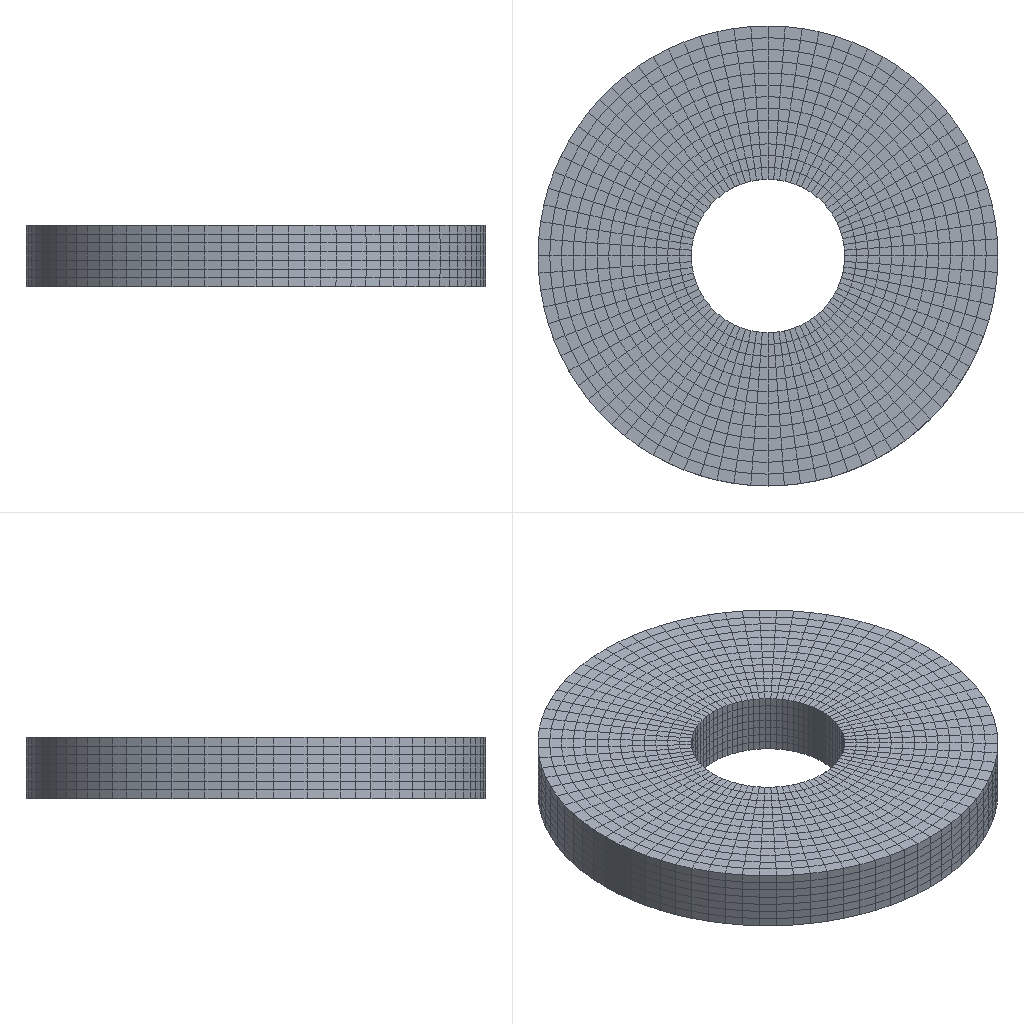Simulation study | abaqus
Set-up summary:
category,name,step,type,value,unit,region
solver,abaqus
solver,version,,,Abaqus/Standard 2020
units,not stated in the deck,,not stated
analysis,deck,,static,static
load_step,Step-1,Step-1,static
load_step,requested,,,1
mesh,nodes,,,10800
mesh,elements,,,9019
element_type,C3D8,,solid,7735
element_type,R3D3,,rigid,14
element_type,R3D4,,rigid,1270
load,load commands in deck,,count,1
bc,support commands in deck,,count,1
material,MATERIAL-1,,in results
material,MATERIAL-1-COPY,,in results
check,setup vs results,,match,"per instance, exact: element labels, types and connectivity; labels of the nodes the elements use; coordinates of those nodes at SINGLE_PRECISION in 2 of 2 instance(s)"
Abaqus input file, long lists of numbers shortened:
*Heading
** Job name: Job-1 Model name: Model-1
** Generated by: Abaqus/CAE 2020
*Preprint, echo=NO, model=NO, history=NO, contact=NO
**
** PARTS
**
*Part, name=Part-1
*Node
      1,   1.118,  -2.236,           4.
      2,   1.118,  -2.236,           0.
** (1277 more lines like these left out)
*Element, type=R3D4
  1,   1,   3, 105, 156
  2,   3,   4, 106, 105
** (1268 more lines like these left out)
*Element, type=R3D3
677,  963,  757,  736
678,  987,  863,  818
** (12 more lines like these left out)
*Node
   1280,           0., -1.5308085e-16,           4.
*Nset, nset=Part-1-RefPt_, internal
1280,
*Elset, elset=Part-1, generate
    1,  1284,     1
*End Part
**
*Part, name=Part-2
*Node
      1,           0.,         -2.5,           2.
      2,           0.,         -7.5,           2.
** (9518 more lines like these left out)
*Element, type=C3D8
   1,    1,   21,  485,   56,   97, 1133, 3689,  886
   2,   21,   22,  486,  485, 1133, 1134, 3690, 3689
** (7733 more lines like these left out)
*Nset, nset=Set-3, generate
    1,  9520,     1
*Elset, elset=Set-3, generate
    1,  7735,     1
** Section: Section-1
*Solid Section, elset=Set-3, material=Material-1
,
*End Part
**
*Part, name=crack2
*End Part
**
**
** ASSEMBLY
**
*Assembly, name=Assembly
**
*Instance, name=Part-1-1, part=Part-1
*End Instance
**
*Instance, name=Part-2-1, part=Part-2
          0.,           0.,           1.
*End Instance
**
*Instance, name=crack2-1, part=crack2
        2.46,         0.05,           2.
*End Instance
**
*Nset, nset=Set-1, instance=Part-1-1
    1,    2,    3,    4,    5,    6,    7,    8,    9,   10,   11,   12,   13,   14,   15,   16
   17,   18,   19,   20,   21,   22,   23,   24,   25,   26,   27,   28,   29,   30,   31,   32
** (39 more lines like these left out)
*Elset, elset=Set-1, instance=Part-1-1, generate
  677,  1284,     1
*Nset, nset=Set-2, instance=Part-1-1
 1280,
*Nset, nset=_PickedSet19, internal, instance=Part-2-1, generate
    1,  9520,     1
*Elset, elset=_PickedSet19, internal, instance=Part-2-1, generate
    1,  7735,     1
*Elset, elset=_Surf-6_S4, internal, instance=Part-2-1, generate
   13,  7735,    13
*Surface, type=ELEMENT, name=Surf-6
_Surf-6_S4, S4
*Elset, elset=_m_Surf-1_SPOS, internal, instance=Part-1-1, generate
   1,  676,    1
*Surface, type=ELEMENT, name=m_Surf-1
_m_Surf-1_SPOS, SPOS
*Elset, elset=_m_Surf-4_SPOS, internal, instance=Part-1-1, generate
   1,  676,    1
*Surface, type=ELEMENT, name=m_Surf-4
_m_Surf-4_SPOS, SPOS
*Elset, elset=_s_Surf-4_S6, internal, instance=Part-2-1, generate
    1,  7723,    13
*Surface, type=ELEMENT, name=s_Surf-4
_s_Surf-4_S6, S6
*Rigid Body, ref node=Part-1-1.Part-1-RefPt_, elset=Part-1-1.Part-1
*Enrichment, name=Crack-1, type=PROPAGATION CRACK, elset=_PickedSet19
*End Assembly
*Amplitude, name=Amp-1
             0.,              0.,              1.,              1.
**
** MATERIALS
**
*Material, name=Material-1
*Damage Initiation, criterion=QUADE, position=CRACKTIP, normal direction=2
 0.001, 0.0001, 0.0001
*Damage Evolution, type=DISPLACEMENT
 1e-08,
*Damage Stabilization
0.0001
*Density
 1e-09,
*Elastic
75800., 0.24
*Material, name=Material-1-Copy
*Damage Initiation, criterion=MAXPS
 0.1,
*Damage Evolution, type=DISPLACEMENT
 1e-06,
*Density
 1e-09,
*Elastic
75800., 0.24
**
** INTERACTION PROPERTIES
**
*Surface Interaction, name=IntProp-1
1.,
*Friction, slip tolerance=0.005
 0.2,
*Surface Behavior, pressure-overclosure=HARD
*Surface Interaction, name=IntProp-2
1.,
*Initial Conditions, type=ENRICHMENT
Part-2-1.195, 1,Crack-1, 0.1429, 0.09689
Part-2-1.195, 2,Crack-1, 0.1429, 0.357
Part-2-1.195, 3,Crack-1, -0.1429, 0.357
Part-2-1.195, 4,Crack-1, -0.1429, 0.09689
Part-2-1.195, 5,Crack-1, 0.1429, -0.03771
Part-2-1.195, 6,Crack-1, 0.1429, 0.204
Part-2-1.195, 7,Crack-1, -0.1429, 0.204
Part-2-1.195, 8,Crack-1, -0.1429, -0.03771
Part-2-1.204, 1,Crack-1, 0.1429, -0.03771
Part-2-1.204, 2,Crack-1, 0.1429, 0.204
Part-2-1.204, 3,Crack-1, -0.1429, 0.204
Part-2-1.204, 4,Crack-1, -0.1429, -0.03771
Part-2-1.204, 5,Crack-1, 0.1429, 0.1032
Part-2-1.204, 6,Crack-1, 0.1429, 0.3666
Part-2-1.204, 7,Crack-1, -0.1429, 0.3666
Part-2-1.204, 8,Crack-1, -0.1429, 0.1032
**
** INTERACTIONS
**
** Interaction: Int-1
*Contact Pair, interaction=IntProp-1, type=SURFACE TO SURFACE
s_Surf-4, m_Surf-4
** ----------------------------------------------------------------
**
** STEP: Step-1
**
*Step, name=Step-1, nlgeom=YES, inc=1000
*Static, stabilize=0.0002, allsdtol=0.05, continue=NO
0.001, 1., 1e-07, 1.
**
** BOUNDARY CONDITIONS
**
** Name: BC-1 Type: 对称/反对称/完全固定
*Boundary
Set-2, ENCASTRE
**
** LOADS
**
** Name: Load-1   Type: Pressure
*Dsload
Surf-6, P, 100.
**
** OUTPUT REQUESTS
**
*Restart, write, frequency=0
**
** FIELD OUTPUT: F-Output-1
**
*Output, field
*Node Output
CF, PHILSM, PSILSM, RF, U, V
*Element Output, directions=YES
E, ENRRTXFEM, LE, MISES, PE, PEEQ, PEMAG, S, SDEG, STATUS, STATUSXFEM
*Contact Output
CDISP, CSTRESS
**
** HISTORY OUTPUT: H-Output-1
**
*Output, history, variable=PRESELECT
*End Step
Results summary:
result,step,,partial,increments=12 time=0.1336/1.0
result,analysis,,,static
result,last_loadstep,,,1
result,primary field,,,U
result,reaction total,,FX,-0.0,model units
result,reaction total,,FY,0.0,model units
result,reaction total,,FZ,0.0,model units